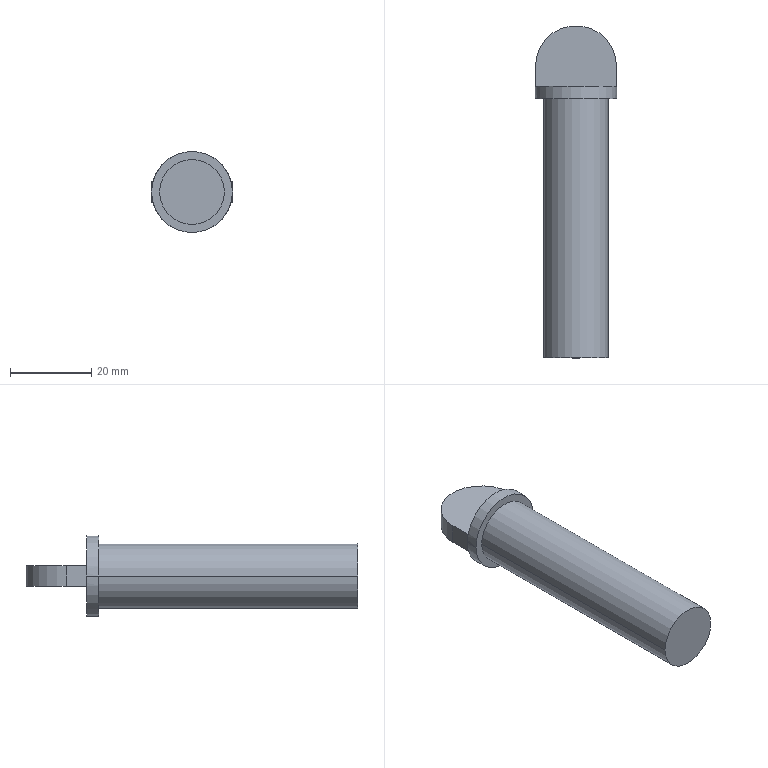Part | STEP file | TNS-16-Part-1 | 1 solid | 17 faces | box 20 x 82 x 20 mm | volume 15096 mm3 | plane 12 | cylinder 5 | commonest cylinder face diameters 20 x3 16 x2
STEP:
#1=CARTESIAN_POINT('',(0.,0.,0.));
#2=DIRECTION('',(0.,0.,1.));
#3=DIRECTION('',(1.,0.,0.));
#4=AXIS2_PLACEMENT_3D('',#1,#2,#3);
#5=CARTESIAN_POINT('',(70.,64.,16.));
#6=VERTEX_POINT('',#5);
#7=CARTESIAN_POINT('',(90.,64.,16.));
#8=VERTEX_POINT('',#7);
#9=CARTESIAN_POINT('',(80.,64.,16.));
#10=DIRECTION('',(0.,1.,0.));
#11=DIRECTION('',(-1.,0.,0.));
#12=AXIS2_PLACEMENT_3D('',#9,#10,#11);
#13=CIRCLE('',#12,10.);
#14=CARTESIAN_POINT('',(80.,64.,16.));
#15=DIRECTION('',(0.,1.,0.));
#16=DIRECTION('',(-1.,0.,0.));
#17=AXIS2_PLACEMENT_3D('',#14,#15,#16);
#18=CYLINDRICAL_SURFACE('',#17,10.);
#19=CARTESIAN_POINT('',(0.,0.));
#20=DIRECTION('',(1.,0.));
#21=VECTOR('',#20,1.);
#22=LINE('',#19,#21);
#23=(GEOMETRIC_REPRESENTATION_CONTEXT(2)PARAMETRIC_REPRESENTATION_CONTEXT()REPRESENTATION_CONTEXT('',''));
#24=DEFINITIONAL_REPRESENTATION('',(#22),#23);
#25=PCURVE('',#18,#24);
#26=CARTESIAN_POINT('',(80.,64.,16.));
#27=DIRECTION('',(0.,-1.,0.));
#28=DIRECTION('',(1.,0.,0.));
#29=AXIS2_PLACEMENT_3D('',#26,#27,#28);
#30=PLANE('',#29);
#31=CARTESIAN_POINT('',(-10.,0.));
#32=CARTESIAN_POINT('',(-10.,17.321));
#33=CARTESIAN_POINT('',(5.,8.66));
#34=CARTESIAN_POINT('',(20.,0.));
#35=CARTESIAN_POINT('',(5.,-8.66));
#36=CARTESIAN_POINT('',(-10.,-17.321));
#37=CARTESIAN_POINT('',(-10.,0.));
#38=(BOUNDED_CURVE()B_SPLINE_CURVE(2,(#31,#32,#33,#34,#35,#36,#37),.UNSPECIFIED.,.T.,.F.)B_SPLINE_CURVE_WITH_KNOTS((1,2,2,2,2,1),(-2.094,0.,2.094,4.189,6.283,8.378),.UNSPECIFIED.)CURVE()GEOMETRIC_REPRESENTATION_ITEM()RATIONAL_B_SPLINE_CURVE((1.,0.5,1.,0.5,1.,0.5,1.))REPRESENTATION_ITEM(''));
#39=(GEOMETRIC_REPRESENTATION_CONTEXT(2)PARAMETRIC_REPRESENTATION_CONTEXT()REPRESENTATION_CONTEXT('',''));
#40=DEFINITIONAL_REPRESENTATION('',(#38),#39);
#41=PCURVE('',#30,#40);
#42=SURFACE_CURVE('',#13,(#25,#41),.PCURVE_S1.);
#43=EDGE_CURVE('',#6,#8,#42,.T.);
#44=ORIENTED_EDGE('',*,*,#43,.T.);
#45=CARTESIAN_POINT('',(90.,67.,16.));
#46=VERTEX_POINT('',#45);
#47=CARTESIAN_POINT('',(90.,64.,16.));
#48=DIRECTION('',(0.,1.,0.));
#49=VECTOR('',#48,1.);
#50=LINE('',#47,#49);
#51=CARTESIAN_POINT('',(3.142,0.));
#52=DIRECTION('',(0.,1.));
#53=VECTOR('',#52,1.);
#54=LINE('',#51,#53);
#55=(GEOMETRIC_REPRESENTATION_CONTEXT(2)PARAMETRIC_REPRESENTATION_CONTEXT()REPRESENTATION_CONTEXT('',''));
#56=DEFINITIONAL_REPRESENTATION('',(#54),#55);
#57=PCURVE('',#18,#56);
#58=CARTESIAN_POINT('',(80.,64.,16.));
#59=DIRECTION('',(0.,1.,0.));
#60=DIRECTION('',(-1.,0.,0.));
#61=AXIS2_PLACEMENT_3D('',#58,#59,#60);
#62=CYLINDRICAL_SURFACE('',#61,10.);
#63=CARTESIAN_POINT('',(3.142,0.));
#64=DIRECTION('',(0.,1.));
#65=VECTOR('',#64,1.);
#66=LINE('',#63,#65);
#67=(GEOMETRIC_REPRESENTATION_CONTEXT(2)PARAMETRIC_REPRESENTATION_CONTEXT()REPRESENTATION_CONTEXT('',''));
#68=DEFINITIONAL_REPRESENTATION('',(#66),#67);
#69=PCURVE('',#62,#68);
#70=SURFACE_CURVE('',#50,(#57,#69),.PCURVE_S1.);
#71=EDGE_CURVE('',#8,#46,#70,.T.);
#72=ORIENTED_EDGE('',*,*,#71,.T.);
#73=CARTESIAN_POINT('',(89.682,67.,18.5));
#74=VERTEX_POINT('',#73);
#75=CARTESIAN_POINT('',(80.,67.,16.));
#76=DIRECTION('',(0.,-1.,0.));
#77=DIRECTION('',(1.,0.,0.));
#78=AXIS2_PLACEMENT_3D('',#75,#76,#77);
#79=CIRCLE('',#78,10.);
#80=CARTESIAN_POINT('',(3.142,3.));
#81=DIRECTION('',(-1.,0.));
#82=VECTOR('',#81,1.);
#83=LINE('',#80,#82);
#84=(GEOMETRIC_REPRESENTATION_CONTEXT(2)PARAMETRIC_REPRESENTATION_CONTEXT()REPRESENTATION_CONTEXT('',''));
#85=DEFINITIONAL_REPRESENTATION('',(#83),#84);
#86=PCURVE('',#18,#85);
#87=CARTESIAN_POINT('',(80.,67.,13.5));
#88=DIRECTION('',(0.,-1.,0.));
#89=DIRECTION('',(0.,0.,1.));
#90=AXIS2_PLACEMENT_3D('',#87,#88,#89);
#91=PLANE('',#90);
#92=CARTESIAN_POINT('',(2.5,0.));
#93=DIRECTION('',(0.,-1.));
#94=AXIS2_PLACEMENT_2D('',#92,#93);
#95=CIRCLE('',#94,10.);
#96=(GEOMETRIC_REPRESENTATION_CONTEXT(2)PARAMETRIC_REPRESENTATION_CONTEXT()REPRESENTATION_CONTEXT('',''));
#97=DEFINITIONAL_REPRESENTATION('',(#95),#96);
#98=PCURVE('',#91,#97);
#99=SURFACE_CURVE('',#79,(#86,#98),.PCURVE_S1.);
#100=EDGE_CURVE('',#46,#74,#99,.T.);
#101=ORIENTED_EDGE('',*,*,#100,.T.);
#102=CARTESIAN_POINT('',(70.318,67.,18.5));
#103=VERTEX_POINT('',#102);
#104=CARTESIAN_POINT('',(80.,67.,16.));
#105=DIRECTION('',(0.,-1.,0.));
#106=DIRECTION('',(1.,0.,0.));
#107=AXIS2_PLACEMENT_3D('',#104,#105,#106);
#108=CIRCLE('',#107,10.);
#109=CARTESIAN_POINT('',(3.142,3.));
#110=DIRECTION('',(-1.,0.));
#111=VECTOR('',#110,1.);
#112=LINE('',#109,#111);
#113=(GEOMETRIC_REPRESENTATION_CONTEXT(2)PARAMETRIC_REPRESENTATION_CONTEXT()REPRESENTATION_CONTEXT('',''));
#114=DEFINITIONAL_REPRESENTATION('',(#112),#113);
#115=PCURVE('',#18,#114);
#116=CARTESIAN_POINT('',(80.,67.,16.));
#117=DIRECTION('',(0.,1.,0.));
#118=DIRECTION('',(-1.,0.,0.));
#119=AXIS2_PLACEMENT_3D('',#116,#117,#118);
#120=PLANE('',#119);
#121=CARTESIAN_POINT('',(-10.,0.));
#122=CARTESIAN_POINT('',(-10.,17.321));
#123=CARTESIAN_POINT('',(5.,8.66));
#124=CARTESIAN_POINT('',(20.,0.));
#125=CARTESIAN_POINT('',(5.,-8.66));
#126=CARTESIAN_POINT('',(-10.,-17.321));
#127=CARTESIAN_POINT('',(-10.,0.));
#128=(BOUNDED_CURVE()B_SPLINE_CURVE(2,(#121,#122,#123,#124,#125,#126,#127),.UNSPECIFIED.,.T.,.F.)B_SPLINE_CURVE_WITH_KNOTS((1,2,2,2,2,1),(-2.094,0.,2.094,4.189,6.283,8.378),.UNSPECIFIED.)CURVE()GEOMETRIC_REPRESENTATION_ITEM()RATIONAL_B_SPLINE_CURVE((1.,0.5,1.,0.5,1.,0.5,1.))REPRESENTATION_ITEM(''));
#129=(GEOMETRIC_REPRESENTATION_CONTEXT(2)PARAMETRIC_REPRESENTATION_CONTEXT()REPRESENTATION_CONTEXT('',''));
#130=DEFINITIONAL_REPRESENTATION('',(#128),#129);
#131=PCURVE('',#120,#130);
#132=SURFACE_CURVE('',#108,(#115,#131),.PCURVE_S1.);
#133=EDGE_CURVE('',#74,#103,#132,.T.);
#134=ORIENTED_EDGE('',*,*,#133,.T.);
#135=CARTESIAN_POINT('',(70.,67.,16.));
#136=VERTEX_POINT('',#135);
#137=CARTESIAN_POINT('',(80.,67.,16.));
#138=DIRECTION('',(0.,-1.,0.));
#139=DIRECTION('',(1.,0.,0.));
#140=AXIS2_PLACEMENT_3D('',#137,#138,#139);
#141=CIRCLE('',#140,10.);
#142=CARTESIAN_POINT('',(3.142,3.));
#143=DIRECTION('',(-1.,0.));
#144=VECTOR('',#143,1.);
#145=LINE('',#142,#144);
#146=(GEOMETRIC_REPRESENTATION_CONTEXT(2)PARAMETRIC_REPRESENTATION_CONTEXT()REPRESENTATION_CONTEXT('',''));
#147=DEFINITIONAL_REPRESENTATION('',(#145),#146);
#148=PCURVE('',#18,#147);
#149=CARTESIAN_POINT('',(80.,67.,13.5));
#150=DIRECTION('',(0.,-1.,0.));
#151=DIRECTION('',(0.,0.,1.));
#152=AXIS2_PLACEMENT_3D('',#149,#150,#151);
#153=PLANE('',#152);
#154=CARTESIAN_POINT('',(2.5,0.));
#155=DIRECTION('',(0.,-1.));
#156=AXIS2_PLACEMENT_2D('',#154,#155);
#157=CIRCLE('',#156,10.);
#158=(GEOMETRIC_REPRESENTATION_CONTEXT(2)PARAMETRIC_REPRESENTATION_CONTEXT()REPRESENTATION_CONTEXT('',''));
#159=DEFINITIONAL_REPRESENTATION('',(#157),#158);
#160=PCURVE('',#153,#159);
#161=SURFACE_CURVE('',#141,(#148,#160),.PCURVE_S1.);
#162=EDGE_CURVE('',#103,#136,#161,.T.);
#163=ORIENTED_EDGE('',*,*,#162,.T.);
#164=CARTESIAN_POINT('',(70.,64.,16.));
#165=DIRECTION('',(0.,1.,0.));
#166=VECTOR('',#165,1.);
#167=LINE('',#164,#166);
#168=CARTESIAN_POINT('',(0.,0.));
#169=DIRECTION('',(0.,1.));
#170=VECTOR('',#169,1.);
#171=LINE('',#168,#170);
#172=(GEOMETRIC_REPRESENTATION_CONTEXT(2)PARAMETRIC_REPRESENTATION_CONTEXT()REPRESENTATION_CONTEXT('',''));
#173=DEFINITIONAL_REPRESENTATION('',(#171),#172);
#174=PCURVE('',#18,#173);
#175=CARTESIAN_POINT('',(6.283,0.));
#176=DIRECTION('',(0.,1.));
#177=VECTOR('',#176,1.);
#178=LINE('',#175,#177);
#179=(GEOMETRIC_REPRESENTATION_CONTEXT(2)PARAMETRIC_REPRESENTATION_CONTEXT()REPRESENTATION_CONTEXT('',''));
#180=DEFINITIONAL_REPRESENTATION('',(#178),#179);
#181=PCURVE('',#62,#180);
#182=SURFACE_CURVE('',#167,(#174,#181),.PCURVE_S1.);
#183=EDGE_CURVE('',#6,#136,#182,.T.);
#184=ORIENTED_EDGE('',*,*,#183,.F.);
#185=EDGE_LOOP('',(#44,#72,#101,#134,#163,#184));
#186=FACE_BOUND('',#185,.T.);
#187=ADVANCED_FACE('',(#186),#18,.T.);
#188=CARTESIAN_POINT('',(72.,0.,16.));
#189=VERTEX_POINT('',#188);
#190=CARTESIAN_POINT('',(88.,0.,16.));
#191=VERTEX_POINT('',#190);
#192=CARTESIAN_POINT('',(80.,0.,16.));
#193=DIRECTION('',(0.,1.,0.));
#194=DIRECTION('',(-1.,0.,0.));
#195=AXIS2_PLACEMENT_3D('',#192,#193,#194);
#196=CIRCLE('',#195,8.);
#197=CARTESIAN_POINT('',(80.,0.,16.));
#198=DIRECTION('',(0.,1.,0.));
#199=DIRECTION('',(-1.,0.,0.));
#200=AXIS2_PLACEMENT_3D('',#197,#198,#199);
#201=CYLINDRICAL_SURFACE('',#200,8.);
#202=CARTESIAN_POINT('',(0.,0.));
#203=DIRECTION('',(1.,0.));
#204=VECTOR('',#203,1.);
#205=LINE('',#202,#204);
#206=(GEOMETRIC_REPRESENTATION_CONTEXT(2)PARAMETRIC_REPRESENTATION_CONTEXT()REPRESENTATION_CONTEXT('',''));
#207=DEFINITIONAL_REPRESENTATION('',(#205),#206);
#208=PCURVE('',#201,#207);
#209=CARTESIAN_POINT('',(80.,0.,16.));
#210=DIRECTION('',(0.,-1.,0.));
#211=DIRECTION('',(1.,0.,0.));
#212=AXIS2_PLACEMENT_3D('',#209,#210,#211);
#213=PLANE('',#212);
#214=CARTESIAN_POINT('',(-8.,0.));
#215=CARTESIAN_POINT('',(-8.,13.856));
#216=CARTESIAN_POINT('',(4.,6.928));
#217=CARTESIAN_POINT('',(16.,0.));
#218=CARTESIAN_POINT('',(4.,-6.928));
#219=CARTESIAN_POINT('',(-8.,-13.856));
#220=CARTESIAN_POINT('',(-8.,0.));
#221=(BOUNDED_CURVE()B_SPLINE_CURVE(2,(#214,#215,#216,#217,#218,#219,#220),.UNSPECIFIED.,.T.,.F.)B_SPLINE_CURVE_WITH_KNOTS((1,2,2,2,2,1),(-2.094,0.,2.094,4.189,6.283,8.378),.UNSPECIFIED.)CURVE()GEOMETRIC_REPRESENTATION_ITEM()RATIONAL_B_SPLINE_CURVE((1.,0.5,1.,0.5,1.,0.5,1.))REPRESENTATION_ITEM(''));
#222=(GEOMETRIC_REPRESENTATION_CONTEXT(2)PARAMETRIC_REPRESENTATION_CONTEXT()REPRESENTATION_CONTEXT('',''));
#223=DEFINITIONAL_REPRESENTATION('',(#221),#222);
#224=PCURVE('',#213,#223);
#225=SURFACE_CURVE('',#196,(#208,#224),.PCURVE_S1.);
#226=EDGE_CURVE('',#189,#191,#225,.T.);
#227=ORIENTED_EDGE('',*,*,#226,.T.);
#228=CARTESIAN_POINT('',(88.,64.,16.));
#229=VERTEX_POINT('',#228);
#230=CARTESIAN_POINT('',(88.,0.,16.));
#231=DIRECTION('',(0.,1.,0.));
#232=VECTOR('',#231,1.);
#233=LINE('',#230,#232);
#234=CARTESIAN_POINT('',(3.142,0.));
#235=DIRECTION('',(0.,1.));
#236=VECTOR('',#235,1.);
#237=LINE('',#234,#236);
#238=(GEOMETRIC_REPRESENTATION_CONTEXT(2)PARAMETRIC_REPRESENTATION_CONTEXT()REPRESENTATION_CONTEXT('',''));
#239=DEFINITIONAL_REPRESENTATION('',(#237),#238);
#240=PCURVE('',#201,#239);
#241=CARTESIAN_POINT('',(80.,0.,16.));
#242=DIRECTION('',(0.,1.,0.));
#243=DIRECTION('',(-1.,0.,0.));
#244=AXIS2_PLACEMENT_3D('',#241,#242,#243);
#245=CYLINDRICAL_SURFACE('',#244,8.);
#246=CARTESIAN_POINT('',(3.142,0.));
#247=DIRECTION('',(0.,1.));
#248=VECTOR('',#247,1.);
#249=LINE('',#246,#248);
#250=(GEOMETRIC_REPRESENTATION_CONTEXT(2)PARAMETRIC_REPRESENTATION_CONTEXT()REPRESENTATION_CONTEXT('',''));
#251=DEFINITIONAL_REPRESENTATION('',(#249),#250);
#252=PCURVE('',#245,#251);
#253=SURFACE_CURVE('',#233,(#240,#252),.PCURVE_S1.);
#254=EDGE_CURVE('',#191,#229,#253,.T.);
#255=ORIENTED_EDGE('',*,*,#254,.T.);
#256=CARTESIAN_POINT('',(72.,64.,16.));
#257=VERTEX_POINT('',#256);
#258=CARTESIAN_POINT('',(80.,64.,16.));
#259=DIRECTION('',(0.,-1.,0.));
#260=DIRECTION('',(1.,0.,0.));
#261=AXIS2_PLACEMENT_3D('',#258,#259,#260);
#262=CIRCLE('',#261,8.);
#263=CARTESIAN_POINT('',(3.142,64.));
#264=DIRECTION('',(-1.,0.));
#265=VECTOR('',#264,1.);
#266=LINE('',#263,#265);
#267=(GEOMETRIC_REPRESENTATION_CONTEXT(2)PARAMETRIC_REPRESENTATION_CONTEXT()REPRESENTATION_CONTEXT('',''));
#268=DEFINITIONAL_REPRESENTATION('',(#266),#267);
#269=PCURVE('',#201,#268);
#270=CARTESIAN_POINT('',(0.,0.));
#271=DIRECTION('',(1.,0.));
#272=AXIS2_PLACEMENT_2D('',#270,#271);
#273=CIRCLE('',#272,8.);
#274=(GEOMETRIC_REPRESENTATION_CONTEXT(2)PARAMETRIC_REPRESENTATION_CONTEXT()REPRESENTATION_CONTEXT('',''));
#275=DEFINITIONAL_REPRESENTATION('',(#273),#274);
#276=PCURVE('',#30,#275);
#277=SURFACE_CURVE('',#262,(#269,#276),.PCURVE_S1.);
#278=EDGE_CURVE('',#229,#257,#277,.T.);
#279=ORIENTED_EDGE('',*,*,#278,.T.);
#280=CARTESIAN_POINT('',(72.,0.,16.));
#281=DIRECTION('',(0.,1.,0.));
#282=VECTOR('',#281,1.);
#283=LINE('',#280,#282);
#284=CARTESIAN_POINT('',(0.,0.));
#285=DIRECTION('',(0.,1.));
#286=VECTOR('',#285,1.);
#287=LINE('',#284,#286);
#288=(GEOMETRIC_REPRESENTATION_CONTEXT(2)PARAMETRIC_REPRESENTATION_CONTEXT()REPRESENTATION_CONTEXT('',''));
#289=DEFINITIONAL_REPRESENTATION('',(#287),#288);
#290=PCURVE('',#201,#289);
#291=CARTESIAN_POINT('',(6.283,0.));
#292=DIRECTION('',(0.,1.));
#293=VECTOR('',#292,1.);
#294=LINE('',#291,#293);
#295=(GEOMETRIC_REPRESENTATION_CONTEXT(2)PARAMETRIC_REPRESENTATION_CONTEXT()REPRESENTATION_CONTEXT('',''));
#296=DEFINITIONAL_REPRESENTATION('',(#294),#295);
#297=PCURVE('',#245,#296);
#298=SURFACE_CURVE('',#283,(#290,#297),.PCURVE_S1.);
#299=EDGE_CURVE('',#189,#257,#298,.T.);
#300=ORIENTED_EDGE('',*,*,#299,.F.);
#301=EDGE_LOOP('',(#227,#255,#279,#300));
#302=FACE_BOUND('',#301,.T.);
#303=ADVANCED_FACE('',(#302),#201,.T.);
#304=ORIENTED_EDGE('',*,*,#226,.F.);
#305=CARTESIAN_POINT('',(80.,0.,16.));
#306=DIRECTION('',(0.,1.,0.));
#307=DIRECTION('',(-1.,0.,0.));
#308=AXIS2_PLACEMENT_3D('',#305,#306,#307);
#309=CIRCLE('',#308,8.);
#310=CARTESIAN_POINT('',(-8.,0.));
#311=CARTESIAN_POINT('',(-8.,13.856));
#312=CARTESIAN_POINT('',(4.,6.928));
#313=CARTESIAN_POINT('',(16.,0.));
#314=CARTESIAN_POINT('',(4.,-6.928));
#315=CARTESIAN_POINT('',(-8.,-13.856));
#316=CARTESIAN_POINT('',(-8.,0.));
#317=(BOUNDED_CURVE()B_SPLINE_CURVE(2,(#310,#311,#312,#313,#314,#315,#316),.UNSPECIFIED.,.T.,.F.)B_SPLINE_CURVE_WITH_KNOTS((1,2,2,2,2,1),(-2.094,0.,2.094,4.189,6.283,8.378),.UNSPECIFIED.)CURVE()GEOMETRIC_REPRESENTATION_ITEM()RATIONAL_B_SPLINE_CURVE((1.,0.5,1.,0.5,1.,0.5,1.))REPRESENTATION_ITEM(''));
#318=(GEOMETRIC_REPRESENTATION_CONTEXT(2)PARAMETRIC_REPRESENTATION_CONTEXT()REPRESENTATION_CONTEXT('',''));
#319=DEFINITIONAL_REPRESENTATION('',(#317),#318);
#320=PCURVE('',#213,#319);
#321=CARTESIAN_POINT('',(0.,0.));
#322=DIRECTION('',(1.,0.));
#323=VECTOR('',#322,1.);
#324=LINE('',#321,#323);
#325=(GEOMETRIC_REPRESENTATION_CONTEXT(2)PARAMETRIC_REPRESENTATION_CONTEXT()REPRESENTATION_CONTEXT('',''));
#326=DEFINITIONAL_REPRESENTATION('',(#324),#325);
#327=PCURVE('',#245,#326);
#328=SURFACE_CURVE('',#309,(#320,#327),.PCURVE_S1.);
#329=EDGE_CURVE('',#191,#189,#328,.T.);
#330=ORIENTED_EDGE('',*,*,#329,.F.);
#331=EDGE_LOOP('',(#304,#330));
#332=FACE_BOUND('',#331,.T.);
#333=ADVANCED_FACE('',(#332),#213,.T.);
#334=ORIENTED_EDGE('',*,*,#254,.F.);
#335=ORIENTED_EDGE('',*,*,#329,.T.);
#336=ORIENTED_EDGE('',*,*,#299,.T.);
#337=CARTESIAN_POINT('',(80.,64.,16.));
#338=DIRECTION('',(0.,-1.,0.));
#339=DIRECTION('',(1.,0.,0.));
#340=AXIS2_PLACEMENT_3D('',#337,#338,#339);
#341=CIRCLE('',#340,8.);
#342=CARTESIAN_POINT('',(9.425,64.));
#343=DIRECTION('',(-1.,0.));
#344=VECTOR('',#343,1.);
#345=LINE('',#342,#344);
#346=(GEOMETRIC_REPRESENTATION_CONTEXT(2)PARAMETRIC_REPRESENTATION_CONTEXT()REPRESENTATION_CONTEXT('',''));
#347=DEFINITIONAL_REPRESENTATION('',(#345),#346);
#348=PCURVE('',#245,#347);
#349=CARTESIAN_POINT('',(0.,0.));
#350=DIRECTION('',(1.,0.));
#351=AXIS2_PLACEMENT_2D('',#349,#350);
#352=CIRCLE('',#351,8.);
#353=(GEOMETRIC_REPRESENTATION_CONTEXT(2)PARAMETRIC_REPRESENTATION_CONTEXT()REPRESENTATION_CONTEXT('',''));
#354=DEFINITIONAL_REPRESENTATION('',(#352),#353);
#355=PCURVE('',#30,#354);
#356=SURFACE_CURVE('',#341,(#348,#355),.PCURVE_S1.);
#357=EDGE_CURVE('',#257,#229,#356,.T.);
#358=ORIENTED_EDGE('',*,*,#357,.T.);
#359=EDGE_LOOP('',(#334,#335,#336,#358));
#360=FACE_BOUND('',#359,.T.);
#361=ADVANCED_FACE('',(#360),#245,.T.);
#362=ORIENTED_EDGE('',*,*,#133,.F.);
#363=CARTESIAN_POINT('',(80.,67.,18.5));
#364=DIRECTION('',(-1.,0.,0.));
#365=VECTOR('',#364,1.);
#366=LINE('',#363,#365);
#367=CARTESIAN_POINT('',(0.,2.5));
#368=DIRECTION('',(1.,0.));
#369=VECTOR('',#368,1.);
#370=LINE('',#367,#369);
#371=(GEOMETRIC_REPRESENTATION_CONTEXT(2)PARAMETRIC_REPRESENTATION_CONTEXT()REPRESENTATION_CONTEXT('',''));
#372=DEFINITIONAL_REPRESENTATION('',(#370),#371);
#373=PCURVE('',#120,#372);
#374=CARTESIAN_POINT('',(80.,74.5,18.5));
#375=DIRECTION('',(0.,0.,1.));
#376=DIRECTION('',(-1.,0.,0.));
#377=AXIS2_PLACEMENT_3D('',#374,#375,#376);
#378=PLANE('',#377);
#379=CARTESIAN_POINT('',(0.,7.5));
#380=DIRECTION('',(1.,0.));
#381=VECTOR('',#380,1.);
#382=LINE('',#379,#381);
#383=(GEOMETRIC_REPRESENTATION_CONTEXT(2)PARAMETRIC_REPRESENTATION_CONTEXT()REPRESENTATION_CONTEXT('',''));
#384=DEFINITIONAL_REPRESENTATION('',(#382),#383);
#385=PCURVE('',#378,#384);
#386=SURFACE_CURVE('',#366,(#373,#385),.PCURVE_S1.);
#387=EDGE_CURVE('',#74,#103,#386,.T.);
#388=ORIENTED_EDGE('',*,*,#387,.T.);
#389=EDGE_LOOP('',(#362,#388));
#390=FACE_BOUND('',#389,.T.);
#391=ADVANCED_FACE('',(#390),#120,.T.);
#392=CARTESIAN_POINT('',(70.318,67.,13.5));
#393=VERTEX_POINT('',#392);
#394=CARTESIAN_POINT('',(89.682,67.,13.5));
#395=VERTEX_POINT('',#394);
#396=CARTESIAN_POINT('',(80.,67.,16.));
#397=DIRECTION('',(0.,-1.,0.));
#398=DIRECTION('',(1.,0.,0.));
#399=AXIS2_PLACEMENT_3D('',#396,#397,#398);
#400=CIRCLE('',#399,10.);
#401=CARTESIAN_POINT('',(80.,67.,16.));
#402=DIRECTION('',(0.,1.,0.));
#403=DIRECTION('',(-1.,0.,0.));
#404=AXIS2_PLACEMENT_3D('',#401,#402,#403);
#405=PLANE('',#404);
#406=CARTESIAN_POINT('',(-10.,0.));
#407=CARTESIAN_POINT('',(-10.,17.321));
#408=CARTESIAN_POINT('',(5.,8.66));
#409=CARTESIAN_POINT('',(20.,0.));
#410=CARTESIAN_POINT('',(5.,-8.66));
#411=CARTESIAN_POINT('',(-10.,-17.321));
#412=CARTESIAN_POINT('',(-10.,0.));
#413=(BOUNDED_CURVE()B_SPLINE_CURVE(2,(#406,#407,#408,#409,#410,#411,#412),.UNSPECIFIED.,.T.,.F.)B_SPLINE_CURVE_WITH_KNOTS((1,2,2,2,2,1),(-2.094,0.,2.094,4.189,6.283,8.378),.UNSPECIFIED.)CURVE()GEOMETRIC_REPRESENTATION_ITEM()RATIONAL_B_SPLINE_CURVE((1.,0.5,1.,0.5,1.,0.5,1.))REPRESENTATION_ITEM(''));
#414=(GEOMETRIC_REPRESENTATION_CONTEXT(2)PARAMETRIC_REPRESENTATION_CONTEXT()REPRESENTATION_CONTEXT('',''));
#415=DEFINITIONAL_REPRESENTATION('',(#413),#414);
#416=PCURVE('',#405,#415);
#417=CARTESIAN_POINT('',(9.425,3.));
#418=DIRECTION('',(-1.,0.));
#419=VECTOR('',#418,1.);
#420=LINE('',#417,#419);
#421=(GEOMETRIC_REPRESENTATION_CONTEXT(2)PARAMETRIC_REPRESENTATION_CONTEXT()REPRESENTATION_CONTEXT('',''));
#422=DEFINITIONAL_REPRESENTATION('',(#420),#421);
#423=PCURVE('',#62,#422);
#424=SURFACE_CURVE('',#400,(#416,#423),.PCURVE_S1.);
#425=EDGE_CURVE('',#393,#395,#424,.T.);
#426=ORIENTED_EDGE('',*,*,#425,.F.);
#427=CARTESIAN_POINT('',(80.,67.,13.5));
#428=DIRECTION('',(1.,0.,0.));
#429=VECTOR('',#428,1.);
#430=LINE('',#427,#429);
#431=CARTESIAN_POINT('',(0.,-2.5));
#432=DIRECTION('',(-1.,0.));
#433=VECTOR('',#432,1.);
#434=LINE('',#431,#433);
#435=(GEOMETRIC_REPRESENTATION_CONTEXT(2)PARAMETRIC_REPRESENTATION_CONTEXT()REPRESENTATION_CONTEXT('',''));
#436=DEFINITIONAL_REPRESENTATION('',(#434),#435);
#437=PCURVE('',#405,#436);
#438=CARTESIAN_POINT('',(80.,74.5,13.5));
#439=DIRECTION('',(0.,0.,-1.));
#440=DIRECTION('',(1.,0.,0.));
#441=AXIS2_PLACEMENT_3D('',#438,#439,#440);
#442=PLANE('',#441);
#443=CARTESIAN_POINT('',(0.,7.5));
#444=DIRECTION('',(1.,0.));
#445=VECTOR('',#444,1.);
#446=LINE('',#443,#445);
#447=(GEOMETRIC_REPRESENTATION_CONTEXT(2)PARAMETRIC_REPRESENTATION_CONTEXT()REPRESENTATION_CONTEXT('',''));
#448=DEFINITIONAL_REPRESENTATION('',(#446),#447);
#449=PCURVE('',#442,#448);
#450=SURFACE_CURVE('',#430,(#437,#449),.PCURVE_S1.);
#451=EDGE_CURVE('',#393,#395,#450,.T.);
#452=ORIENTED_EDGE('',*,*,#451,.T.);
#453=EDGE_LOOP('',(#426,#452));
#454=FACE_BOUND('',#453,.T.);
#455=ADVANCED_FACE('',(#454),#405,.T.);
#456=ORIENTED_EDGE('',*,*,#357,.F.);
#457=ORIENTED_EDGE('',*,*,#278,.F.);
#458=EDGE_LOOP('',(#456,#457));
#459=FACE_BOUND('',#458,.T.);
#460=ORIENTED_EDGE('',*,*,#43,.F.);
#461=CARTESIAN_POINT('',(80.,64.,16.));
#462=DIRECTION('',(0.,1.,0.));
#463=DIRECTION('',(-1.,0.,0.));
#464=AXIS2_PLACEMENT_3D('',#461,#462,#463);
#465=CIRCLE('',#464,10.);
#466=CARTESIAN_POINT('',(-10.,0.));
#467=CARTESIAN_POINT('',(-10.,17.321));
#468=CARTESIAN_POINT('',(5.,8.66));
#469=CARTESIAN_POINT('',(20.,0.));
#470=CARTESIAN_POINT('',(5.,-8.66));
#471=CARTESIAN_POINT('',(-10.,-17.321));
#472=CARTESIAN_POINT('',(-10.,0.));
#473=(BOUNDED_CURVE()B_SPLINE_CURVE(2,(#466,#467,#468,#469,#470,#471,#472),.UNSPECIFIED.,.T.,.F.)B_SPLINE_CURVE_WITH_KNOTS((1,2,2,2,2,1),(-2.094,0.,2.094,4.189,6.283,8.378),.UNSPECIFIED.)CURVE()GEOMETRIC_REPRESENTATION_ITEM()RATIONAL_B_SPLINE_CURVE((1.,0.5,1.,0.5,1.,0.5,1.))REPRESENTATION_ITEM(''));
#474=(GEOMETRIC_REPRESENTATION_CONTEXT(2)PARAMETRIC_REPRESENTATION_CONTEXT()REPRESENTATION_CONTEXT('',''));
#475=DEFINITIONAL_REPRESENTATION('',(#473),#474);
#476=PCURVE('',#30,#475);
#477=CARTESIAN_POINT('',(0.,0.));
#478=DIRECTION('',(1.,0.));
#479=VECTOR('',#478,1.);
#480=LINE('',#477,#479);
#481=(GEOMETRIC_REPRESENTATION_CONTEXT(2)PARAMETRIC_REPRESENTATION_CONTEXT()REPRESENTATION_CONTEXT('',''));
#482=DEFINITIONAL_REPRESENTATION('',(#480),#481);
#483=PCURVE('',#62,#482);
#484=SURFACE_CURVE('',#465,(#476,#483),.PCURVE_S1.);
#485=EDGE_CURVE('',#8,#6,#484,.T.);
#486=ORIENTED_EDGE('',*,*,#485,.F.);
#487=EDGE_LOOP('',(#460,#486));
#488=FACE_BOUND('',#487,.T.);
#489=ADVANCED_FACE('',(#459,#488),#30,.T.);
#490=ORIENTED_EDGE('',*,*,#71,.F.);
#491=ORIENTED_EDGE('',*,*,#485,.T.);
#492=ORIENTED_EDGE('',*,*,#183,.T.);
#493=CARTESIAN_POINT('',(80.,67.,16.));
#494=DIRECTION('',(0.,-1.,0.));
#495=DIRECTION('',(1.,0.,0.));
#496=AXIS2_PLACEMENT_3D('',#493,#494,#495);
#497=CIRCLE('',#496,10.);
#498=CARTESIAN_POINT('',(9.425,3.));
#499=DIRECTION('',(-1.,0.));
#500=VECTOR('',#499,1.);
#501=LINE('',#498,#500);
#502=(GEOMETRIC_REPRESENTATION_CONTEXT(2)PARAMETRIC_REPRESENTATION_CONTEXT()REPRESENTATION_CONTEXT('',''));
#503=DEFINITIONAL_REPRESENTATION('',(#501),#502);
#504=PCURVE('',#62,#503);
#505=CARTESIAN_POINT('',(80.,67.,13.5));
#506=DIRECTION('',(0.,-1.,0.));
#507=DIRECTION('',(0.,0.,1.));
#508=AXIS2_PLACEMENT_3D('',#505,#506,#507);
#509=PLANE('',#508);
#510=CARTESIAN_POINT('',(2.5,0.));
#511=DIRECTION('',(0.,-1.));
#512=AXIS2_PLACEMENT_2D('',#510,#511);
#513=CIRCLE('',#512,10.);
#514=(GEOMETRIC_REPRESENTATION_CONTEXT(2)PARAMETRIC_REPRESENTATION_CONTEXT()REPRESENTATION_CONTEXT('',''));
#515=DEFINITIONAL_REPRESENTATION('',(#513),#514);
#516=PCURVE('',#509,#515);
#517=SURFACE_CURVE('',#497,(#504,#516),.PCURVE_S1.);
#518=EDGE_CURVE('',#136,#393,#517,.T.);
#519=ORIENTED_EDGE('',*,*,#518,.T.);
#520=ORIENTED_EDGE('',*,*,#425,.T.);
#521=CARTESIAN_POINT('',(80.,67.,16.));
#522=DIRECTION('',(0.,-1.,0.));
#523=DIRECTION('',(1.,0.,0.));
#524=AXIS2_PLACEMENT_3D('',#521,#522,#523);
#525=CIRCLE('',#524,10.);
#526=CARTESIAN_POINT('',(9.425,3.));
#527=DIRECTION('',(-1.,0.));
#528=VECTOR('',#527,1.);
#529=LINE('',#526,#528);
#530=(GEOMETRIC_REPRESENTATION_CONTEXT(2)PARAMETRIC_REPRESENTATION_CONTEXT()REPRESENTATION_CONTEXT('',''));
#531=DEFINITIONAL_REPRESENTATION('',(#529),#530);
#532=PCURVE('',#62,#531);
#533=CARTESIAN_POINT('',(80.,67.,13.5));
#534=DIRECTION('',(0.,-1.,0.));
#535=DIRECTION('',(0.,0.,1.));
#536=AXIS2_PLACEMENT_3D('',#533,#534,#535);
#537=PLANE('',#536);
#538=CARTESIAN_POINT('',(2.5,0.));
#539=DIRECTION('',(0.,-1.));
#540=AXIS2_PLACEMENT_2D('',#538,#539);
#541=CIRCLE('',#540,10.);
#542=(GEOMETRIC_REPRESENTATION_CONTEXT(2)PARAMETRIC_REPRESENTATION_CONTEXT()REPRESENTATION_CONTEXT('',''));
#543=DEFINITIONAL_REPRESENTATION('',(#541),#542);
#544=PCURVE('',#537,#543);
#545=SURFACE_CURVE('',#525,(#532,#544),.PCURVE_S1.);
#546=EDGE_CURVE('',#395,#46,#545,.T.);
#547=ORIENTED_EDGE('',*,*,#546,.T.);
#548=EDGE_LOOP('',(#490,#491,#492,#519,#520,#547));
#549=FACE_BOUND('',#548,.T.);
#550=ADVANCED_FACE('',(#549),#62,.T.);
#551=ORIENTED_EDGE('',*,*,#162,.F.);
#552=CARTESIAN_POINT('',(70.,67.,18.5));
#553=VERTEX_POINT('',#552);
#554=CARTESIAN_POINT('',(80.,67.,18.5));
#555=DIRECTION('',(-1.,0.,0.));
#556=VECTOR('',#555,1.);
#557=LINE('',#554,#556);
#558=CARTESIAN_POINT('',(5.,0.));
#559=DIRECTION('',(0.,1.));
#560=VECTOR('',#559,1.);
#561=LINE('',#558,#560);
#562=(GEOMETRIC_REPRESENTATION_CONTEXT(2)PARAMETRIC_REPRESENTATION_CONTEXT()REPRESENTATION_CONTEXT('',''));
#563=DEFINITIONAL_REPRESENTATION('',(#561),#562);
#564=PCURVE('',#153,#563);
#565=CARTESIAN_POINT('',(0.,7.5));
#566=DIRECTION('',(1.,0.));
#567=VECTOR('',#566,1.);
#568=LINE('',#565,#567);
#569=(GEOMETRIC_REPRESENTATION_CONTEXT(2)PARAMETRIC_REPRESENTATION_CONTEXT()REPRESENTATION_CONTEXT('',''));
#570=DEFINITIONAL_REPRESENTATION('',(#568),#569);
#571=PCURVE('',#378,#570);
#572=SURFACE_CURVE('',#557,(#564,#571),.PCURVE_S1.);
#573=EDGE_CURVE('',#103,#553,#572,.T.);
#574=ORIENTED_EDGE('',*,*,#573,.T.);
#575=CARTESIAN_POINT('',(70.,67.,13.5));
#576=DIRECTION('',(0.,0.,1.));
#577=VECTOR('',#576,1.);
#578=LINE('',#575,#577);
#579=CARTESIAN_POINT('',(0.,10.));
#580=DIRECTION('',(1.,0.));
#581=VECTOR('',#580,1.);
#582=LINE('',#579,#581);
#583=(GEOMETRIC_REPRESENTATION_CONTEXT(2)PARAMETRIC_REPRESENTATION_CONTEXT()REPRESENTATION_CONTEXT('',''));
#584=DEFINITIONAL_REPRESENTATION('',(#582),#583);
#585=PCURVE('',#153,#584);
#586=CARTESIAN_POINT('',(70.,74.5,13.5));
#587=DIRECTION('',(-1.,0.,0.));
#588=DIRECTION('',(0.,0.,-1.));
#589=AXIS2_PLACEMENT_3D('',#586,#587,#588);
#590=PLANE('',#589);
#591=CARTESIAN_POINT('',(0.,7.5));
#592=DIRECTION('',(-1.,0.));
#593=VECTOR('',#592,1.);
#594=LINE('',#591,#593);
#595=(GEOMETRIC_REPRESENTATION_CONTEXT(2)PARAMETRIC_REPRESENTATION_CONTEXT()REPRESENTATION_CONTEXT('',''));
#596=DEFINITIONAL_REPRESENTATION('',(#594),#595);
#597=PCURVE('',#590,#596);
#598=SURFACE_CURVE('',#578,(#585,#597),.PCURVE_S1.);
#599=EDGE_CURVE('',#136,#553,#598,.T.);
#600=ORIENTED_EDGE('',*,*,#599,.F.);
#601=EDGE_LOOP('',(#551,#574,#600));
#602=FACE_BOUND('',#601,.T.);
#603=ADVANCED_FACE('',(#602),#153,.T.);
#604=ORIENTED_EDGE('',*,*,#518,.F.);
#605=CARTESIAN_POINT('',(70.,67.,13.5));
#606=VERTEX_POINT('',#605);
#607=CARTESIAN_POINT('',(70.,67.,13.5));
#608=DIRECTION('',(0.,0.,1.));
#609=VECTOR('',#608,1.);
#610=LINE('',#607,#609);
#611=CARTESIAN_POINT('',(0.,10.));
#612=DIRECTION('',(1.,0.));
#613=VECTOR('',#612,1.);
#614=LINE('',#611,#613);
#615=(GEOMETRIC_REPRESENTATION_CONTEXT(2)PARAMETRIC_REPRESENTATION_CONTEXT()REPRESENTATION_CONTEXT('',''));
#616=DEFINITIONAL_REPRESENTATION('',(#614),#615);
#617=PCURVE('',#509,#616);
#618=CARTESIAN_POINT('',(0.,7.5));
#619=DIRECTION('',(-1.,0.));
#620=VECTOR('',#619,1.);
#621=LINE('',#618,#620);
#622=(GEOMETRIC_REPRESENTATION_CONTEXT(2)PARAMETRIC_REPRESENTATION_CONTEXT()REPRESENTATION_CONTEXT('',''));
#623=DEFINITIONAL_REPRESENTATION('',(#621),#622);
#624=PCURVE('',#590,#623);
#625=SURFACE_CURVE('',#610,(#617,#624),.PCURVE_S1.);
#626=EDGE_CURVE('',#606,#136,#625,.T.);
#627=ORIENTED_EDGE('',*,*,#626,.F.);
#628=CARTESIAN_POINT('',(80.,67.,13.5));
#629=DIRECTION('',(1.,0.,0.));
#630=VECTOR('',#629,1.);
#631=LINE('',#628,#630);
#632=CARTESIAN_POINT('',(0.,0.));
#633=DIRECTION('',(0.,-1.));
#634=VECTOR('',#633,1.);
#635=LINE('',#632,#634);
#636=(GEOMETRIC_REPRESENTATION_CONTEXT(2)PARAMETRIC_REPRESENTATION_CONTEXT()REPRESENTATION_CONTEXT('',''));
#637=DEFINITIONAL_REPRESENTATION('',(#635),#636);
#638=PCURVE('',#509,#637);
#639=CARTESIAN_POINT('',(0.,7.5));
#640=DIRECTION('',(1.,0.));
#641=VECTOR('',#640,1.);
#642=LINE('',#639,#641);
#643=(GEOMETRIC_REPRESENTATION_CONTEXT(2)PARAMETRIC_REPRESENTATION_CONTEXT()REPRESENTATION_CONTEXT('',''));
#644=DEFINITIONAL_REPRESENTATION('',(#642),#643);
#645=PCURVE('',#442,#644);
#646=SURFACE_CURVE('',#631,(#638,#645),.PCURVE_S1.);
#647=EDGE_CURVE('',#606,#393,#646,.T.);
#648=ORIENTED_EDGE('',*,*,#647,.T.);
#649=EDGE_LOOP('',(#604,#627,#648));
#650=FACE_BOUND('',#649,.T.);
#651=ADVANCED_FACE('',(#650),#509,.T.);
#652=ORIENTED_EDGE('',*,*,#100,.F.);
#653=CARTESIAN_POINT('',(90.,67.,18.5));
#654=VERTEX_POINT('',#653);
#655=CARTESIAN_POINT('',(90.,67.,13.5));
#656=DIRECTION('',(0.,0.,1.));
#657=VECTOR('',#656,1.);
#658=LINE('',#655,#657);
#659=CARTESIAN_POINT('',(0.,-10.));
#660=DIRECTION('',(1.,0.));
#661=VECTOR('',#660,1.);
#662=LINE('',#659,#661);
#663=(GEOMETRIC_REPRESENTATION_CONTEXT(2)PARAMETRIC_REPRESENTATION_CONTEXT()REPRESENTATION_CONTEXT('',''));
#664=DEFINITIONAL_REPRESENTATION('',(#662),#663);
#665=PCURVE('',#91,#664);
#666=CARTESIAN_POINT('',(90.,74.5,13.5));
#667=DIRECTION('',(1.,0.,0.));
#668=DIRECTION('',(0.,0.,1.));
#669=AXIS2_PLACEMENT_3D('',#666,#667,#668);
#670=PLANE('',#669);
#671=CARTESIAN_POINT('',(0.,7.5));
#672=DIRECTION('',(1.,0.));
#673=VECTOR('',#672,1.);
#674=LINE('',#671,#673);
#675=(GEOMETRIC_REPRESENTATION_CONTEXT(2)PARAMETRIC_REPRESENTATION_CONTEXT()REPRESENTATION_CONTEXT('',''));
#676=DEFINITIONAL_REPRESENTATION('',(#674),#675);
#677=PCURVE('',#670,#676);
#678=SURFACE_CURVE('',#658,(#665,#677),.PCURVE_S1.);
#679=EDGE_CURVE('',#46,#654,#678,.T.);
#680=ORIENTED_EDGE('',*,*,#679,.T.);
#681=CARTESIAN_POINT('',(80.,67.,18.5));
#682=DIRECTION('',(-1.,0.,0.));
#683=VECTOR('',#682,1.);
#684=LINE('',#681,#683);
#685=CARTESIAN_POINT('',(5.,0.));
#686=DIRECTION('',(0.,1.));
#687=VECTOR('',#686,1.);
#688=LINE('',#685,#687);
#689=(GEOMETRIC_REPRESENTATION_CONTEXT(2)PARAMETRIC_REPRESENTATION_CONTEXT()REPRESENTATION_CONTEXT('',''));
#690=DEFINITIONAL_REPRESENTATION('',(#688),#689);
#691=PCURVE('',#91,#690);
#692=CARTESIAN_POINT('',(0.,7.5));
#693=DIRECTION('',(1.,0.));
#694=VECTOR('',#693,1.);
#695=LINE('',#692,#694);
#696=(GEOMETRIC_REPRESENTATION_CONTEXT(2)PARAMETRIC_REPRESENTATION_CONTEXT()REPRESENTATION_CONTEXT('',''));
#697=DEFINITIONAL_REPRESENTATION('',(#695),#696);
#698=PCURVE('',#378,#697);
#699=SURFACE_CURVE('',#684,(#691,#698),.PCURVE_S1.);
#700=EDGE_CURVE('',#654,#74,#699,.T.);
#701=ORIENTED_EDGE('',*,*,#700,.T.);
#702=EDGE_LOOP('',(#652,#680,#701));
#703=FACE_BOUND('',#702,.T.);
#704=ADVANCED_FACE('',(#703),#91,.T.);
#705=ORIENTED_EDGE('',*,*,#546,.F.);
#706=CARTESIAN_POINT('',(90.,67.,13.5));
#707=VERTEX_POINT('',#706);
#708=CARTESIAN_POINT('',(80.,67.,13.5));
#709=DIRECTION('',(1.,0.,0.));
#710=VECTOR('',#709,1.);
#711=LINE('',#708,#710);
#712=CARTESIAN_POINT('',(0.,0.));
#713=DIRECTION('',(0.,-1.));
#714=VECTOR('',#713,1.);
#715=LINE('',#712,#714);
#716=(GEOMETRIC_REPRESENTATION_CONTEXT(2)PARAMETRIC_REPRESENTATION_CONTEXT()REPRESENTATION_CONTEXT('',''));
#717=DEFINITIONAL_REPRESENTATION('',(#715),#716);
#718=PCURVE('',#537,#717);
#719=CARTESIAN_POINT('',(0.,7.5));
#720=DIRECTION('',(1.,0.));
#721=VECTOR('',#720,1.);
#722=LINE('',#719,#721);
#723=(GEOMETRIC_REPRESENTATION_CONTEXT(2)PARAMETRIC_REPRESENTATION_CONTEXT()REPRESENTATION_CONTEXT('',''));
#724=DEFINITIONAL_REPRESENTATION('',(#722),#723);
#725=PCURVE('',#442,#724);
#726=SURFACE_CURVE('',#711,(#718,#725),.PCURVE_S1.);
#727=EDGE_CURVE('',#395,#707,#726,.T.);
#728=ORIENTED_EDGE('',*,*,#727,.T.);
#729=CARTESIAN_POINT('',(90.,67.,13.5));
#730=DIRECTION('',(0.,0.,1.));
#731=VECTOR('',#730,1.);
#732=LINE('',#729,#731);
#733=CARTESIAN_POINT('',(0.,-10.));
#734=DIRECTION('',(1.,0.));
#735=VECTOR('',#734,1.);
#736=LINE('',#733,#735);
#737=(GEOMETRIC_REPRESENTATION_CONTEXT(2)PARAMETRIC_REPRESENTATION_CONTEXT()REPRESENTATION_CONTEXT('',''));
#738=DEFINITIONAL_REPRESENTATION('',(#736),#737);
#739=PCURVE('',#537,#738);
#740=CARTESIAN_POINT('',(0.,7.5));
#741=DIRECTION('',(1.,0.));
#742=VECTOR('',#741,1.);
#743=LINE('',#740,#742);
#744=(GEOMETRIC_REPRESENTATION_CONTEXT(2)PARAMETRIC_REPRESENTATION_CONTEXT()REPRESENTATION_CONTEXT('',''));
#745=DEFINITIONAL_REPRESENTATION('',(#743),#744);
#746=PCURVE('',#670,#745);
#747=SURFACE_CURVE('',#732,(#739,#746),.PCURVE_S1.);
#748=EDGE_CURVE('',#707,#46,#747,.T.);
#749=ORIENTED_EDGE('',*,*,#748,.T.);
#750=EDGE_LOOP('',(#705,#728,#749));
#751=FACE_BOUND('',#750,.T.);
#752=ADVANCED_FACE('',(#751),#537,.T.);
#753=CARTESIAN_POINT('',(90.,72.,18.5));
#754=VERTEX_POINT('',#753);
#755=CARTESIAN_POINT('',(90.,74.5,18.5));
#756=DIRECTION('',(0.,-1.,0.));
#757=VECTOR('',#756,1.);
#758=LINE('',#755,#757);
#759=CARTESIAN_POINT('',(-10.,0.));
#760=DIRECTION('',(0.,1.));
#761=VECTOR('',#760,1.);
#762=LINE('',#759,#761);
#763=(GEOMETRIC_REPRESENTATION_CONTEXT(2)PARAMETRIC_REPRESENTATION_CONTEXT()REPRESENTATION_CONTEXT('',''));
#764=DEFINITIONAL_REPRESENTATION('',(#762),#763);
#765=PCURVE('',#378,#764);
#766=CARTESIAN_POINT('',(5.,0.));
#767=DIRECTION('',(0.,1.));
#768=VECTOR('',#767,1.);
#769=LINE('',#766,#768);
#770=(GEOMETRIC_REPRESENTATION_CONTEXT(2)PARAMETRIC_REPRESENTATION_CONTEXT()REPRESENTATION_CONTEXT('',''));
#771=DEFINITIONAL_REPRESENTATION('',(#769),#770);
#772=PCURVE('',#670,#771);
#773=SURFACE_CURVE('',#758,(#765,#772),.PCURVE_S1.);
#774=EDGE_CURVE('',#754,#654,#773,.T.);
#775=ORIENTED_EDGE('',*,*,#774,.F.);
#776=CARTESIAN_POINT('',(70.,72.,18.5));
#777=VERTEX_POINT('',#776);
#778=CARTESIAN_POINT('',(80.,72.,18.5));
#779=DIRECTION('',(0.,0.,1.));
#780=DIRECTION('',(-1.,0.,0.));
#781=AXIS2_PLACEMENT_3D('',#778,#779,#780);
#782=CIRCLE('',#781,10.);
#783=CARTESIAN_POINT('',(0.,2.5));
#784=DIRECTION('',(1.,0.));
#785=AXIS2_PLACEMENT_2D('',#783,#784);
#786=CIRCLE('',#785,10.);
#787=(GEOMETRIC_REPRESENTATION_CONTEXT(2)PARAMETRIC_REPRESENTATION_CONTEXT()REPRESENTATION_CONTEXT('',''));
#788=DEFINITIONAL_REPRESENTATION('',(#786),#787);
#789=PCURVE('',#378,#788);
#790=CARTESIAN_POINT('',(80.,72.,13.5));
#791=DIRECTION('',(0.,0.,1.));
#792=DIRECTION('',(-1.,0.,0.));
#793=AXIS2_PLACEMENT_3D('',#790,#791,#792);
#794=CYLINDRICAL_SURFACE('',#793,10.);
#795=CARTESIAN_POINT('',(0.,5.));
#796=DIRECTION('',(1.,0.));
#797=VECTOR('',#796,1.);
#798=LINE('',#795,#797);
#799=(GEOMETRIC_REPRESENTATION_CONTEXT(2)PARAMETRIC_REPRESENTATION_CONTEXT()REPRESENTATION_CONTEXT('',''));
#800=DEFINITIONAL_REPRESENTATION('',(#798),#799);
#801=PCURVE('',#794,#800);
#802=SURFACE_CURVE('',#782,(#789,#801),.PCURVE_S1.);
#803=EDGE_CURVE('',#754,#777,#802,.T.);
#804=ORIENTED_EDGE('',*,*,#803,.T.);
#805=CARTESIAN_POINT('',(70.,74.5,18.5));
#806=DIRECTION('',(0.,1.,0.));
#807=VECTOR('',#806,1.);
#808=LINE('',#805,#807);
#809=CARTESIAN_POINT('',(10.,0.));
#810=DIRECTION('',(0.,-1.));
#811=VECTOR('',#810,1.);
#812=LINE('',#809,#811);
#813=(GEOMETRIC_REPRESENTATION_CONTEXT(2)PARAMETRIC_REPRESENTATION_CONTEXT()REPRESENTATION_CONTEXT('',''));
#814=DEFINITIONAL_REPRESENTATION('',(#812),#813);
#815=PCURVE('',#378,#814);
#816=CARTESIAN_POINT('',(-5.,0.));
#817=DIRECTION('',(0.,-1.));
#818=VECTOR('',#817,1.);
#819=LINE('',#816,#818);
#820=(GEOMETRIC_REPRESENTATION_CONTEXT(2)PARAMETRIC_REPRESENTATION_CONTEXT()REPRESENTATION_CONTEXT('',''));
#821=DEFINITIONAL_REPRESENTATION('',(#819),#820);
#822=PCURVE('',#590,#821);
#823=SURFACE_CURVE('',#808,(#815,#822),.PCURVE_S1.);
#824=EDGE_CURVE('',#553,#777,#823,.T.);
#825=ORIENTED_EDGE('',*,*,#824,.F.);
#826=ORIENTED_EDGE('',*,*,#573,.F.);
#827=ORIENTED_EDGE('',*,*,#387,.F.);
#828=ORIENTED_EDGE('',*,*,#700,.F.);
#829=EDGE_LOOP('',(#775,#804,#825,#826,#827,#828));
#830=FACE_BOUND('',#829,.T.);
#831=ADVANCED_FACE('',(#830),#378,.T.);
#832=CARTESIAN_POINT('',(90.,72.,13.5));
#833=VERTEX_POINT('',#832);
#834=CARTESIAN_POINT('',(90.,74.5,13.5));
#835=DIRECTION('',(0.,1.,0.));
#836=VECTOR('',#835,1.);
#837=LINE('',#834,#836);
#838=CARTESIAN_POINT('',(0.,0.));
#839=DIRECTION('',(0.,-1.));
#840=VECTOR('',#839,1.);
#841=LINE('',#838,#840);
#842=(GEOMETRIC_REPRESENTATION_CONTEXT(2)PARAMETRIC_REPRESENTATION_CONTEXT()REPRESENTATION_CONTEXT('',''));
#843=DEFINITIONAL_REPRESENTATION('',(#841),#842);
#844=PCURVE('',#670,#843);
#845=CARTESIAN_POINT('',(10.,0.));
#846=DIRECTION('',(0.,-1.));
#847=VECTOR('',#846,1.);
#848=LINE('',#845,#847);
#849=(GEOMETRIC_REPRESENTATION_CONTEXT(2)PARAMETRIC_REPRESENTATION_CONTEXT()REPRESENTATION_CONTEXT('',''));
#850=DEFINITIONAL_REPRESENTATION('',(#848),#849);
#851=PCURVE('',#442,#850);
#852=SURFACE_CURVE('',#837,(#844,#851),.PCURVE_S1.);
#853=EDGE_CURVE('',#707,#833,#852,.T.);
#854=ORIENTED_EDGE('',*,*,#853,.T.);
#855=CARTESIAN_POINT('',(90.,72.,13.5));
#856=DIRECTION('',(0.,0.,1.));
#857=VECTOR('',#856,1.);
#858=LINE('',#855,#857);
#859=CARTESIAN_POINT('',(0.,2.5));
#860=DIRECTION('',(1.,0.));
#861=VECTOR('',#860,1.);
#862=LINE('',#859,#861);
#863=(GEOMETRIC_REPRESENTATION_CONTEXT(2)PARAMETRIC_REPRESENTATION_CONTEXT()REPRESENTATION_CONTEXT('',''));
#864=DEFINITIONAL_REPRESENTATION('',(#862),#863);
#865=PCURVE('',#670,#864);
#866=CARTESIAN_POINT('',(3.142,0.));
#867=DIRECTION('',(0.,1.));
#868=VECTOR('',#867,1.);
#869=LINE('',#866,#868);
#870=(GEOMETRIC_REPRESENTATION_CONTEXT(2)PARAMETRIC_REPRESENTATION_CONTEXT()REPRESENTATION_CONTEXT('',''));
#871=DEFINITIONAL_REPRESENTATION('',(#869),#870);
#872=PCURVE('',#794,#871);
#873=SURFACE_CURVE('',#858,(#865,#872),.PCURVE_S1.);
#874=EDGE_CURVE('',#833,#754,#873,.T.);
#875=ORIENTED_EDGE('',*,*,#874,.T.);
#876=ORIENTED_EDGE('',*,*,#774,.T.);
#877=ORIENTED_EDGE('',*,*,#679,.F.);
#878=ORIENTED_EDGE('',*,*,#748,.F.);
#879=EDGE_LOOP('',(#854,#875,#876,#877,#878));
#880=FACE_BOUND('',#879,.T.);
#881=ADVANCED_FACE('',(#880),#670,.T.);
#882=CARTESIAN_POINT('',(70.,72.,13.5));
#883=VERTEX_POINT('',#882);
#884=CARTESIAN_POINT('',(80.,72.,13.5));
#885=DIRECTION('',(0.,0.,-1.));
#886=DIRECTION('',(1.,0.,0.));
#887=AXIS2_PLACEMENT_3D('',#884,#885,#886);
#888=CIRCLE('',#887,10.);
#889=CARTESIAN_POINT('',(0.,2.5));
#890=DIRECTION('',(1.,0.));
#891=AXIS2_PLACEMENT_2D('',#889,#890);
#892=CIRCLE('',#891,10.);
#893=(GEOMETRIC_REPRESENTATION_CONTEXT(2)PARAMETRIC_REPRESENTATION_CONTEXT()REPRESENTATION_CONTEXT('',''));
#894=DEFINITIONAL_REPRESENTATION('',(#892),#893);
#895=PCURVE('',#442,#894);
#896=CARTESIAN_POINT('',(9.425,0.));
#897=DIRECTION('',(-1.,0.));
#898=VECTOR('',#897,1.);
#899=LINE('',#896,#898);
#900=(GEOMETRIC_REPRESENTATION_CONTEXT(2)PARAMETRIC_REPRESENTATION_CONTEXT()REPRESENTATION_CONTEXT('',''));
#901=DEFINITIONAL_REPRESENTATION('',(#899),#900);
#902=PCURVE('',#794,#901);
#903=SURFACE_CURVE('',#888,(#895,#902),.PCURVE_S1.);
#904=EDGE_CURVE('',#883,#833,#903,.T.);
#905=ORIENTED_EDGE('',*,*,#904,.T.);
#906=ORIENTED_EDGE('',*,*,#853,.F.);
#907=ORIENTED_EDGE('',*,*,#727,.F.);
#908=ORIENTED_EDGE('',*,*,#451,.F.);
#909=ORIENTED_EDGE('',*,*,#647,.F.);
#910=CARTESIAN_POINT('',(70.,74.5,13.5));
#911=DIRECTION('',(0.,-1.,0.));
#912=VECTOR('',#911,1.);
#913=LINE('',#910,#912);
#914=CARTESIAN_POINT('',(-10.,0.));
#915=DIRECTION('',(0.,1.));
#916=VECTOR('',#915,1.);
#917=LINE('',#914,#916);
#918=(GEOMETRIC_REPRESENTATION_CONTEXT(2)PARAMETRIC_REPRESENTATION_CONTEXT()REPRESENTATION_CONTEXT('',''));
#919=DEFINITIONAL_REPRESENTATION('',(#917),#918);
#920=PCURVE('',#442,#919);
#921=CARTESIAN_POINT('',(0.,0.));
#922=DIRECTION('',(0.,1.));
#923=VECTOR('',#922,1.);
#924=LINE('',#921,#923);
#925=(GEOMETRIC_REPRESENTATION_CONTEXT(2)PARAMETRIC_REPRESENTATION_CONTEXT()REPRESENTATION_CONTEXT('',''));
#926=DEFINITIONAL_REPRESENTATION('',(#924),#925);
#927=PCURVE('',#590,#926);
#928=SURFACE_CURVE('',#913,(#920,#927),.PCURVE_S1.);
#929=EDGE_CURVE('',#883,#606,#928,.T.);
#930=ORIENTED_EDGE('',*,*,#929,.F.);
#931=EDGE_LOOP('',(#905,#906,#907,#908,#909,#930));
#932=FACE_BOUND('',#931,.T.);
#933=ADVANCED_FACE('',(#932),#442,.T.);
#934=ORIENTED_EDGE('',*,*,#824,.T.);
#935=CARTESIAN_POINT('',(70.,72.,13.5));
#936=DIRECTION('',(0.,0.,-1.));
#937=VECTOR('',#936,1.);
#938=LINE('',#935,#937);
#939=CARTESIAN_POINT('',(0.,2.5));
#940=DIRECTION('',(1.,0.));
#941=VECTOR('',#940,1.);
#942=LINE('',#939,#941);
#943=(GEOMETRIC_REPRESENTATION_CONTEXT(2)PARAMETRIC_REPRESENTATION_CONTEXT()REPRESENTATION_CONTEXT('',''));
#944=DEFINITIONAL_REPRESENTATION('',(#942),#943);
#945=PCURVE('',#590,#944);
#946=CARTESIAN_POINT('',(6.283,0.));
#947=DIRECTION('',(0.,-1.));
#948=VECTOR('',#947,1.);
#949=LINE('',#946,#948);
#950=(GEOMETRIC_REPRESENTATION_CONTEXT(2)PARAMETRIC_REPRESENTATION_CONTEXT()REPRESENTATION_CONTEXT('',''));
#951=DEFINITIONAL_REPRESENTATION('',(#949),#950);
#952=PCURVE('',#794,#951);
#953=SURFACE_CURVE('',#938,(#945,#952),.PCURVE_S1.);
#954=EDGE_CURVE('',#777,#883,#953,.T.);
#955=ORIENTED_EDGE('',*,*,#954,.T.);
#956=ORIENTED_EDGE('',*,*,#929,.T.);
#957=ORIENTED_EDGE('',*,*,#626,.T.);
#958=ORIENTED_EDGE('',*,*,#599,.T.);
#959=EDGE_LOOP('',(#934,#955,#956,#957,#958));
#960=FACE_BOUND('',#959,.T.);
#961=ADVANCED_FACE('',(#960),#590,.T.);
#962=ORIENTED_EDGE('',*,*,#904,.F.);
#963=ORIENTED_EDGE('',*,*,#954,.F.);
#964=ORIENTED_EDGE('',*,*,#803,.F.);
#965=ORIENTED_EDGE('',*,*,#874,.F.);
#966=EDGE_LOOP('',(#962,#963,#964,#965));
#967=FACE_BOUND('',#966,.T.);
#968=ADVANCED_FACE('',(#967),#794,.T.);
#969=CLOSED_SHELL('',(#187,#303,#333,#361,#391,#455,#489,#550,#603,#651,#704,#752,#831,#881,#933,#961,#968));
#970=MANIFOLD_SOLID_BREP('',#969);
#971=(LENGTH_UNIT()NAMED_UNIT(*)SI_UNIT(.MILLI.,.METRE.));
#972=UNCERTAINTY_MEASURE_WITH_UNIT(LENGTH_MEASURE(0.0000001),#971,'','');
#973=(NAMED_UNIT(*)PLANE_ANGLE_UNIT()SI_UNIT($,.RADIAN.));
#974=(NAMED_UNIT(*)SI_UNIT($,.STERADIAN.)SOLID_ANGLE_UNIT());
#975=(GEOMETRIC_REPRESENTATION_CONTEXT(3)GLOBAL_UNCERTAINTY_ASSIGNED_CONTEXT((#972))GLOBAL_UNIT_ASSIGNED_CONTEXT((#971,#973,#974))REPRESENTATION_CONTEXT('',''));
#976=ADVANCED_BREP_SHAPE_REPRESENTATION('',(#4,#970),#975);